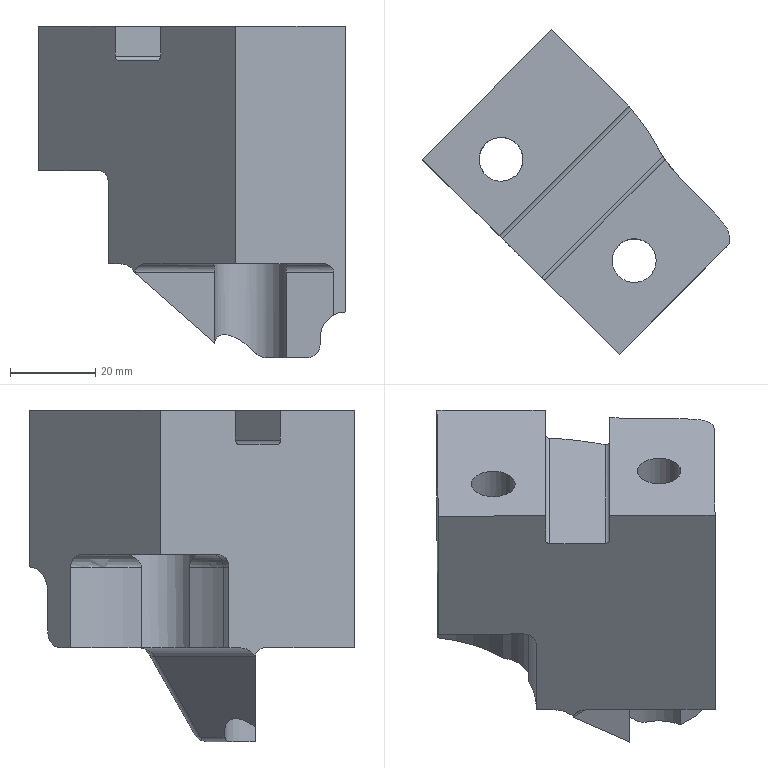Part | NX | features solid 2 | 1 solid | 56 faces | box 71.88 x 76.2 x 77.75 mm | volume 122411 mm3 | plane 23 | cylinder 21 | spline 9 | torus 3 | commonest cylinder face diameters 6 x4 12 x3 2 x2 4 x2 8 x2 10.3 x2